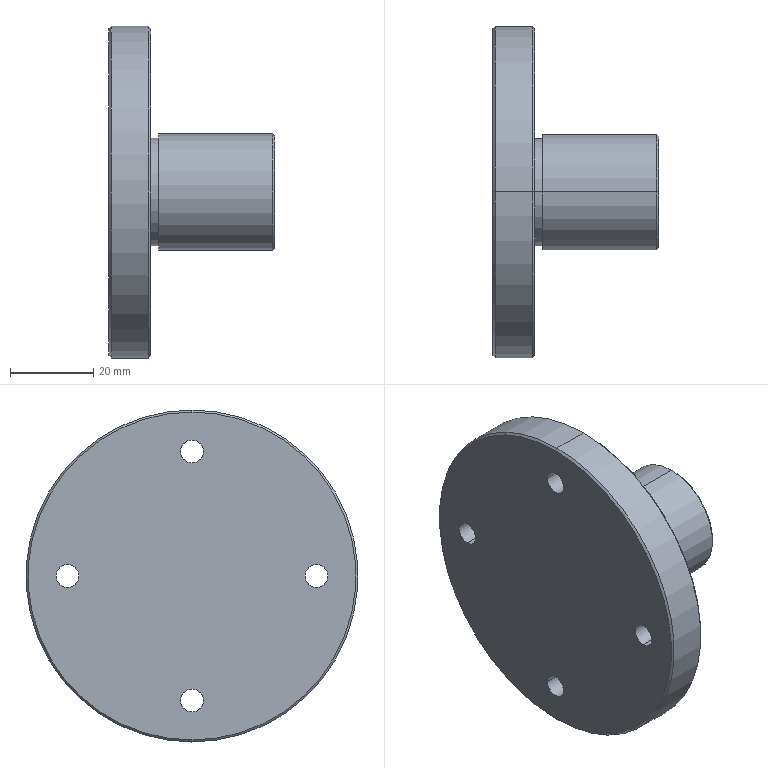Part | SolidWorks | features HoleWzd 2, Chamfer 1, CirPattern 1, ICE 1, Revolution 1 | 1 solid | 36 faces | box 40 x 80 x 80 mm | volume 66296 mm3 | cylinder 22 | plane 8 | cone 6 | commonest cylinder face diameters 5.5 x8 10 x8 26 x2 28 x2 80 x2
STEP:
#1=CARTESIAN_POINT('',(4.3,-30.,-5.));
#2=VERTEX_POINT('',#1);
#3=CARTESIAN_POINT('',(4.3,-30.,5.));
#4=VERTEX_POINT('',#3);
#5=CARTESIAN_POINT('',(4.3,-30.,0.));
#6=DIRECTION('',(1.,0.,0.));
#7=DIRECTION('',(0.,0.,1.));
#8=AXIS2_PLACEMENT_3D('',#5,#6,#7);
#9=CIRCLE('',#8,5.);
#10=EDGE_CURVE('',#2,#4,#9,.T.);
#11=ORIENTED_EDGE('',*,*,#10,.F.);
#12=CARTESIAN_POINT('',(10.,-30.,-5.));
#13=VERTEX_POINT('',#12);
#14=CARTESIAN_POINT('',(10.,-30.,-5.));
#15=DIRECTION('',(1.,0.,0.));
#16=VECTOR('',#15,1000.);
#17=LINE('',#14,#16);
#18=EDGE_CURVE('',#2,#13,#17,.T.);
#19=ORIENTED_EDGE('',*,*,#18,.T.);
#20=CARTESIAN_POINT('',(10.,-30.,5.));
#21=VERTEX_POINT('',#20);
#22=CARTESIAN_POINT('',(10.,-30.,0.));
#23=DIRECTION('',(1.,0.,0.));
#24=DIRECTION('',(0.,0.,1.));
#25=AXIS2_PLACEMENT_3D('',#22,#23,#24);
#26=CIRCLE('',#25,5.);
#27=EDGE_CURVE('',#13,#21,#26,.T.);
#28=ORIENTED_EDGE('',*,*,#27,.T.);
#29=CARTESIAN_POINT('',(10.,-30.,5.));
#30=DIRECTION('',(1.,0.,0.));
#31=VECTOR('',#30,1000.);
#32=LINE('',#29,#31);
#33=EDGE_CURVE('',#4,#21,#32,.T.);
#34=ORIENTED_EDGE('',*,*,#33,.F.);
#35=EDGE_LOOP('',(#11,#19,#28,#34));
#36=FACE_OUTER_BOUND('',#35,.T.);
#37=CARTESIAN_POINT('',(10.,-30.,0.));
#38=DIRECTION('',(1.,0.,0.));
#39=DIRECTION('',(0.,0.,1.));
#40=AXIS2_PLACEMENT_3D('',#37,#38,#39);
#41=CYLINDRICAL_SURFACE('',#40,5.);
#42=ADVANCED_FACE('',(#36),#41,.F.);
#43=CARTESIAN_POINT('',(0.,-30.,-2.75));
#44=VERTEX_POINT('',#43);
#45=CARTESIAN_POINT('',(0.,-30.,2.75));
#46=VERTEX_POINT('',#45);
#47=CARTESIAN_POINT('',(0.,-30.,0.));
#48=DIRECTION('',(1.,0.,0.));
#49=DIRECTION('',(0.,0.,1.));
#50=AXIS2_PLACEMENT_3D('',#47,#48,#49);
#51=CIRCLE('',#50,2.75);
#52=EDGE_CURVE('',#44,#46,#51,.T.);
#53=ORIENTED_EDGE('',*,*,#52,.F.);
#54=CARTESIAN_POINT('',(4.3,-30.,-2.75));
#55=VERTEX_POINT('',#54);
#56=CARTESIAN_POINT('',(10.,-30.,-2.75));
#57=DIRECTION('',(1.,0.,0.));
#58=VECTOR('',#57,1000.);
#59=LINE('',#56,#58);
#60=EDGE_CURVE('',#44,#55,#59,.T.);
#61=ORIENTED_EDGE('',*,*,#60,.T.);
#62=CARTESIAN_POINT('',(4.3,-30.,2.75));
#63=VERTEX_POINT('',#62);
#64=CARTESIAN_POINT('',(4.3,-30.,0.));
#65=DIRECTION('',(1.,0.,0.));
#66=DIRECTION('',(0.,0.,1.));
#67=AXIS2_PLACEMENT_3D('',#64,#65,#66);
#68=CIRCLE('',#67,2.75);
#69=EDGE_CURVE('',#55,#63,#68,.T.);
#70=ORIENTED_EDGE('',*,*,#69,.T.);
#71=CARTESIAN_POINT('',(10.,-30.,2.75));
#72=DIRECTION('',(1.,0.,0.));
#73=VECTOR('',#72,1000.);
#74=LINE('',#71,#73);
#75=EDGE_CURVE('',#46,#63,#74,.T.);
#76=ORIENTED_EDGE('',*,*,#75,.F.);
#77=EDGE_LOOP('',(#53,#61,#70,#76));
#78=FACE_OUTER_BOUND('',#77,.T.);
#79=CARTESIAN_POINT('',(10.,-30.,0.));
#80=DIRECTION('',(1.,0.,0.));
#81=DIRECTION('',(0.,0.,1.));
#82=AXIS2_PLACEMENT_3D('',#79,#80,#81);
#83=CYLINDRICAL_SURFACE('',#82,2.75);
#84=ADVANCED_FACE('',(#78),#83,.F.);
#85=CARTESIAN_POINT('',(4.3,5.,-30.));
#86=VERTEX_POINT('',#85);
#87=CARTESIAN_POINT('',(4.3,-5.,-30.));
#88=VERTEX_POINT('',#87);
#89=CARTESIAN_POINT('',(4.3,0.,-30.));
#90=DIRECTION('',(1.,0.,0.));
#91=DIRECTION('',(0.,-1.,0.));
#92=AXIS2_PLACEMENT_3D('',#89,#90,#91);
#93=CIRCLE('',#92,5.);
#94=EDGE_CURVE('',#86,#88,#93,.T.);
#95=ORIENTED_EDGE('',*,*,#94,.F.);
#96=CARTESIAN_POINT('',(10.,5.,-30.));
#97=VERTEX_POINT('',#96);
#98=CARTESIAN_POINT('',(10.,5.,-30.));
#99=DIRECTION('',(1.,0.,0.));
#100=VECTOR('',#99,1000.);
#101=LINE('',#98,#100);
#102=EDGE_CURVE('',#86,#97,#101,.T.);
#103=ORIENTED_EDGE('',*,*,#102,.T.);
#104=CARTESIAN_POINT('',(10.,-5.,-30.));
#105=VERTEX_POINT('',#104);
#106=CARTESIAN_POINT('',(10.,0.,-30.));
#107=DIRECTION('',(1.,0.,0.));
#108=DIRECTION('',(0.,-1.,0.));
#109=AXIS2_PLACEMENT_3D('',#106,#107,#108);
#110=CIRCLE('',#109,5.);
#111=EDGE_CURVE('',#97,#105,#110,.T.);
#112=ORIENTED_EDGE('',*,*,#111,.T.);
#113=CARTESIAN_POINT('',(10.,-5.,-30.));
#114=DIRECTION('',(1.,0.,0.));
#115=VECTOR('',#114,1000.);
#116=LINE('',#113,#115);
#117=EDGE_CURVE('',#88,#105,#116,.T.);
#118=ORIENTED_EDGE('',*,*,#117,.F.);
#119=EDGE_LOOP('',(#95,#103,#112,#118));
#120=FACE_OUTER_BOUND('',#119,.T.);
#121=CARTESIAN_POINT('',(10.,0.,-30.));
#122=DIRECTION('',(1.,0.,0.));
#123=DIRECTION('',(0.,-1.,0.));
#124=AXIS2_PLACEMENT_3D('',#121,#122,#123);
#125=CYLINDRICAL_SURFACE('',#124,5.);
#126=ADVANCED_FACE('',(#120),#125,.F.);
#127=CARTESIAN_POINT('',(0.,2.75,-30.));
#128=VERTEX_POINT('',#127);
#129=CARTESIAN_POINT('',(0.,-2.75,-30.));
#130=VERTEX_POINT('',#129);
#131=CARTESIAN_POINT('',(0.,0.,-30.));
#132=DIRECTION('',(1.,0.,0.));
#133=DIRECTION('',(0.,-1.,0.));
#134=AXIS2_PLACEMENT_3D('',#131,#132,#133);
#135=CIRCLE('',#134,2.75);
#136=EDGE_CURVE('',#128,#130,#135,.T.);
#137=ORIENTED_EDGE('',*,*,#136,.F.);
#138=CARTESIAN_POINT('',(4.3,2.75,-30.));
#139=VERTEX_POINT('',#138);
#140=CARTESIAN_POINT('',(10.,2.75,-30.));
#141=DIRECTION('',(1.,0.,0.));
#142=VECTOR('',#141,1000.);
#143=LINE('',#140,#142);
#144=EDGE_CURVE('',#128,#139,#143,.T.);
#145=ORIENTED_EDGE('',*,*,#144,.T.);
#146=CARTESIAN_POINT('',(4.3,-2.75,-30.));
#147=VERTEX_POINT('',#146);
#148=CARTESIAN_POINT('',(4.3,0.,-30.));
#149=DIRECTION('',(1.,0.,0.));
#150=DIRECTION('',(0.,-1.,0.));
#151=AXIS2_PLACEMENT_3D('',#148,#149,#150);
#152=CIRCLE('',#151,2.75);
#153=EDGE_CURVE('',#139,#147,#152,.T.);
#154=ORIENTED_EDGE('',*,*,#153,.T.);
#155=CARTESIAN_POINT('',(10.,-2.75,-30.));
#156=DIRECTION('',(1.,0.,0.));
#157=VECTOR('',#156,1000.);
#158=LINE('',#155,#157);
#159=EDGE_CURVE('',#130,#147,#158,.T.);
#160=ORIENTED_EDGE('',*,*,#159,.F.);
#161=EDGE_LOOP('',(#137,#145,#154,#160));
#162=FACE_OUTER_BOUND('',#161,.T.);
#163=CARTESIAN_POINT('',(10.,0.,-30.));
#164=DIRECTION('',(1.,0.,0.));
#165=DIRECTION('',(0.,-1.,0.));
#166=AXIS2_PLACEMENT_3D('',#163,#164,#165);
#167=CYLINDRICAL_SURFACE('',#166,2.75);
#168=ADVANCED_FACE('',(#162),#167,.F.);
#169=CARTESIAN_POINT('',(4.3,-5.,30.));
#170=VERTEX_POINT('',#169);
#171=CARTESIAN_POINT('',(4.3,5.,30.));
#172=VERTEX_POINT('',#171);
#173=CARTESIAN_POINT('',(4.3,0.,30.));
#174=DIRECTION('',(1.,0.,0.));
#175=DIRECTION('',(0.,1.,0.));
#176=AXIS2_PLACEMENT_3D('',#173,#174,#175);
#177=CIRCLE('',#176,5.);
#178=EDGE_CURVE('',#170,#172,#177,.T.);
#179=ORIENTED_EDGE('',*,*,#178,.F.);
#180=CARTESIAN_POINT('',(10.,-5.,30.));
#181=VERTEX_POINT('',#180);
#182=CARTESIAN_POINT('',(10.,-5.,30.));
#183=DIRECTION('',(1.,0.,0.));
#184=VECTOR('',#183,1000.);
#185=LINE('',#182,#184);
#186=EDGE_CURVE('',#170,#181,#185,.T.);
#187=ORIENTED_EDGE('',*,*,#186,.T.);
#188=CARTESIAN_POINT('',(10.,5.,30.));
#189=VERTEX_POINT('',#188);
#190=CARTESIAN_POINT('',(10.,0.,30.));
#191=DIRECTION('',(1.,0.,0.));
#192=DIRECTION('',(0.,1.,0.));
#193=AXIS2_PLACEMENT_3D('',#190,#191,#192);
#194=CIRCLE('',#193,5.);
#195=EDGE_CURVE('',#181,#189,#194,.T.);
#196=ORIENTED_EDGE('',*,*,#195,.T.);
#197=CARTESIAN_POINT('',(10.,5.,30.));
#198=DIRECTION('',(1.,0.,0.));
#199=VECTOR('',#198,1000.);
#200=LINE('',#197,#199);
#201=EDGE_CURVE('',#172,#189,#200,.T.);
#202=ORIENTED_EDGE('',*,*,#201,.F.);
#203=EDGE_LOOP('',(#179,#187,#196,#202));
#204=FACE_OUTER_BOUND('',#203,.T.);
#205=CARTESIAN_POINT('',(10.,0.,30.));
#206=DIRECTION('',(1.,0.,0.));
#207=DIRECTION('',(0.,1.,0.));
#208=AXIS2_PLACEMENT_3D('',#205,#206,#207);
#209=CYLINDRICAL_SURFACE('',#208,5.);
#210=ADVANCED_FACE('',(#204),#209,.F.);
#211=CARTESIAN_POINT('',(0.,-2.75,30.));
#212=VERTEX_POINT('',#211);
#213=CARTESIAN_POINT('',(0.,2.75,30.));
#214=VERTEX_POINT('',#213);
#215=CARTESIAN_POINT('',(0.,0.,30.));
#216=DIRECTION('',(1.,0.,0.));
#217=DIRECTION('',(0.,1.,0.));
#218=AXIS2_PLACEMENT_3D('',#215,#216,#217);
#219=CIRCLE('',#218,2.75);
#220=EDGE_CURVE('',#212,#214,#219,.T.);
#221=ORIENTED_EDGE('',*,*,#220,.F.);
#222=CARTESIAN_POINT('',(4.3,-2.75,30.));
#223=VERTEX_POINT('',#222);
#224=CARTESIAN_POINT('',(10.,-2.75,30.));
#225=DIRECTION('',(1.,0.,0.));
#226=VECTOR('',#225,1000.);
#227=LINE('',#224,#226);
#228=EDGE_CURVE('',#212,#223,#227,.T.);
#229=ORIENTED_EDGE('',*,*,#228,.T.);
#230=CARTESIAN_POINT('',(4.3,2.75,30.));
#231=VERTEX_POINT('',#230);
#232=CARTESIAN_POINT('',(4.3,0.,30.));
#233=DIRECTION('',(1.,0.,0.));
#234=DIRECTION('',(0.,1.,0.));
#235=AXIS2_PLACEMENT_3D('',#232,#233,#234);
#236=CIRCLE('',#235,2.75);
#237=EDGE_CURVE('',#223,#231,#236,.T.);
#238=ORIENTED_EDGE('',*,*,#237,.T.);
#239=CARTESIAN_POINT('',(10.,2.75,30.));
#240=DIRECTION('',(1.,0.,0.));
#241=VECTOR('',#240,1000.);
#242=LINE('',#239,#241);
#243=EDGE_CURVE('',#214,#231,#242,.T.);
#244=ORIENTED_EDGE('',*,*,#243,.F.);
#245=EDGE_LOOP('',(#221,#229,#238,#244));
#246=FACE_OUTER_BOUND('',#245,.T.);
#247=CARTESIAN_POINT('',(10.,0.,30.));
#248=DIRECTION('',(1.,0.,0.));
#249=DIRECTION('',(0.,1.,0.));
#250=AXIS2_PLACEMENT_3D('',#247,#248,#249);
#251=CYLINDRICAL_SURFACE('',#250,2.75);
#252=ADVANCED_FACE('',(#246),#251,.F.);
#253=CARTESIAN_POINT('',(4.3,30.,5.));
#254=VERTEX_POINT('',#253);
#255=CARTESIAN_POINT('',(4.3,30.,-5.));
#256=VERTEX_POINT('',#255);
#257=CARTESIAN_POINT('',(4.3,30.,0.));
#258=DIRECTION('',(1.,0.,0.));
#259=DIRECTION('',(0.,0.,-1.));
#260=AXIS2_PLACEMENT_3D('',#257,#258,#259);
#261=CIRCLE('',#260,5.);
#262=EDGE_CURVE('',#254,#256,#261,.T.);
#263=ORIENTED_EDGE('',*,*,#262,.F.);
#264=CARTESIAN_POINT('',(10.,30.,5.));
#265=VERTEX_POINT('',#264);
#266=CARTESIAN_POINT('',(10.,30.,5.));
#267=DIRECTION('',(1.,0.,0.));
#268=VECTOR('',#267,1000.);
#269=LINE('',#266,#268);
#270=EDGE_CURVE('',#254,#265,#269,.T.);
#271=ORIENTED_EDGE('',*,*,#270,.T.);
#272=CARTESIAN_POINT('',(10.,30.,-5.));
#273=VERTEX_POINT('',#272);
#274=CARTESIAN_POINT('',(10.,30.,0.));
#275=DIRECTION('',(1.,0.,0.));
#276=DIRECTION('',(0.,0.,-1.));
#277=AXIS2_PLACEMENT_3D('',#274,#275,#276);
#278=CIRCLE('',#277,5.);
#279=EDGE_CURVE('',#265,#273,#278,.T.);
#280=ORIENTED_EDGE('',*,*,#279,.T.);
#281=CARTESIAN_POINT('',(10.,30.,-5.));
#282=DIRECTION('',(1.,0.,0.));
#283=VECTOR('',#282,1000.);
#284=LINE('',#281,#283);
#285=EDGE_CURVE('',#256,#273,#284,.T.);
#286=ORIENTED_EDGE('',*,*,#285,.F.);
#287=EDGE_LOOP('',(#263,#271,#280,#286));
#288=FACE_OUTER_BOUND('',#287,.T.);
#289=CARTESIAN_POINT('',(10.,30.,0.));
#290=DIRECTION('',(1.,0.,0.));
#291=DIRECTION('',(0.,0.,-1.));
#292=AXIS2_PLACEMENT_3D('',#289,#290,#291);
#293=CYLINDRICAL_SURFACE('',#292,5.);
#294=ADVANCED_FACE('',(#288),#293,.F.);
#295=CARTESIAN_POINT('',(0.,30.,2.75));
#296=VERTEX_POINT('',#295);
#297=CARTESIAN_POINT('',(0.,30.,-2.75));
#298=VERTEX_POINT('',#297);
#299=CARTESIAN_POINT('',(0.,30.,0.));
#300=DIRECTION('',(1.,0.,0.));
#301=DIRECTION('',(0.,0.,-1.));
#302=AXIS2_PLACEMENT_3D('',#299,#300,#301);
#303=CIRCLE('',#302,2.75);
#304=EDGE_CURVE('',#296,#298,#303,.T.);
#305=ORIENTED_EDGE('',*,*,#304,.F.);
#306=CARTESIAN_POINT('',(4.3,30.,2.75));
#307=VERTEX_POINT('',#306);
#308=CARTESIAN_POINT('',(10.,30.,2.75));
#309=DIRECTION('',(1.,0.,0.));
#310=VECTOR('',#309,1000.);
#311=LINE('',#308,#310);
#312=EDGE_CURVE('',#296,#307,#311,.T.);
#313=ORIENTED_EDGE('',*,*,#312,.T.);
#314=CARTESIAN_POINT('',(4.3,30.,-2.75));
#315=VERTEX_POINT('',#314);
#316=CARTESIAN_POINT('',(4.3,30.,0.));
#317=DIRECTION('',(1.,0.,0.));
#318=DIRECTION('',(0.,0.,-1.));
#319=AXIS2_PLACEMENT_3D('',#316,#317,#318);
#320=CIRCLE('',#319,2.75);
#321=EDGE_CURVE('',#307,#315,#320,.T.);
#322=ORIENTED_EDGE('',*,*,#321,.T.);
#323=CARTESIAN_POINT('',(10.,30.,-2.75));
#324=DIRECTION('',(1.,0.,0.));
#325=VECTOR('',#324,1000.);
#326=LINE('',#323,#325);
#327=EDGE_CURVE('',#298,#315,#326,.T.);
#328=ORIENTED_EDGE('',*,*,#327,.F.);
#329=EDGE_LOOP('',(#305,#313,#322,#328));
#330=FACE_OUTER_BOUND('',#329,.T.);
#331=CARTESIAN_POINT('',(10.,30.,0.));
#332=DIRECTION('',(1.,0.,0.));
#333=DIRECTION('',(0.,0.,-1.));
#334=AXIS2_PLACEMENT_3D('',#331,#332,#333);
#335=CYLINDRICAL_SURFACE('',#334,2.75);
#336=ADVANCED_FACE('',(#330),#335,.F.);
#337=CARTESIAN_POINT('',(40.,0.,-13.5));
#338=VERTEX_POINT('',#337);
#339=CARTESIAN_POINT('',(40.,0.,13.5));
#340=VERTEX_POINT('',#339);
#341=CARTESIAN_POINT('',(40.,0.,0.));
#342=DIRECTION('',(1.,0.,0.));
#343=DIRECTION('',(0.,0.,1.));
#344=AXIS2_PLACEMENT_3D('',#341,#342,#343);
#345=CIRCLE('',#344,13.5);
#346=EDGE_CURVE('',#338,#340,#345,.T.);
#347=ORIENTED_EDGE('',*,*,#346,.F.);
#348=CARTESIAN_POINT('',(39.5,0.,-14.));
#349=VERTEX_POINT('',#348);
#350=CARTESIAN_POINT('',(39.5,0.,-14.));
#351=DIRECTION('',(-0.7071,0.,-0.7071));
#352=VECTOR('',#351,1000.);
#353=LINE('',#350,#352);
#354=EDGE_CURVE('',#338,#349,#353,.T.);
#355=ORIENTED_EDGE('',*,*,#354,.T.);
#356=CARTESIAN_POINT('',(39.5,0.,14.));
#357=VERTEX_POINT('',#356);
#358=CARTESIAN_POINT('',(39.5,0.,0.));
#359=DIRECTION('',(-1.,0.,0.));
#360=DIRECTION('',(0.,0.,1.));
#361=AXIS2_PLACEMENT_3D('',#358,#359,#360);
#362=CIRCLE('',#361,14.);
#363=EDGE_CURVE('',#357,#349,#362,.T.);
#364=ORIENTED_EDGE('',*,*,#363,.F.);
#365=CARTESIAN_POINT('',(39.5,0.,14.));
#366=DIRECTION('',(-0.7071,0.,0.7071));
#367=VECTOR('',#366,1000.);
#368=LINE('',#365,#367);
#369=EDGE_CURVE('',#340,#357,#368,.T.);
#370=ORIENTED_EDGE('',*,*,#369,.F.);
#371=EDGE_LOOP('',(#347,#355,#364,#370));
#372=FACE_OUTER_BOUND('',#371,.T.);
#373=CARTESIAN_POINT('',(39.5,0.,0.));
#374=DIRECTION('',(-1.,0.,0.));
#375=DIRECTION('',(0.,0.,1.));
#376=AXIS2_PLACEMENT_3D('',#373,#374,#375);
#377=CONICAL_SURFACE('',#376,14.,0.7854);
#378=ADVANCED_FACE('',(#372),#377,.T.);
#379=CARTESIAN_POINT('',(0.,0.,39.5));
#380=VERTEX_POINT('',#379);
#381=CARTESIAN_POINT('',(0.,0.,-39.5));
#382=VERTEX_POINT('',#381);
#383=CARTESIAN_POINT('',(0.,0.,0.));
#384=DIRECTION('',(-1.,0.,0.));
#385=DIRECTION('',(0.,0.,-1.));
#386=AXIS2_PLACEMENT_3D('',#383,#384,#385);
#387=CIRCLE('',#386,39.5);
#388=EDGE_CURVE('',#380,#382,#387,.T.);
#389=ORIENTED_EDGE('',*,*,#388,.F.);
#390=CARTESIAN_POINT('',(0.5,0.,40.));
#391=VERTEX_POINT('',#390);
#392=CARTESIAN_POINT('',(0.,0.,39.5));
#393=DIRECTION('',(0.7071,0.,0.7071));
#394=VECTOR('',#393,1000.);
#395=LINE('',#392,#394);
#396=EDGE_CURVE('',#380,#391,#395,.T.);
#397=ORIENTED_EDGE('',*,*,#396,.T.);
#398=CARTESIAN_POINT('',(0.5,0.,-40.));
#399=VERTEX_POINT('',#398);
#400=CARTESIAN_POINT('',(0.5,0.,0.));
#401=DIRECTION('',(1.,0.,0.));
#402=DIRECTION('',(0.,0.,-1.));
#403=AXIS2_PLACEMENT_3D('',#400,#401,#402);
#404=CIRCLE('',#403,40.);
#405=EDGE_CURVE('',#399,#391,#404,.T.);
#406=ORIENTED_EDGE('',*,*,#405,.F.);
#407=CARTESIAN_POINT('',(0.,0.,-39.5));
#408=DIRECTION('',(0.7071,0.,-0.7071));
#409=VECTOR('',#408,1000.);
#410=LINE('',#407,#409);
#411=EDGE_CURVE('',#382,#399,#410,.T.);
#412=ORIENTED_EDGE('',*,*,#411,.F.);
#413=EDGE_LOOP('',(#389,#397,#406,#412));
#414=FACE_OUTER_BOUND('',#413,.T.);
#415=CARTESIAN_POINT('',(0.,0.,0.));
#416=DIRECTION('',(1.,0.,0.));
#417=DIRECTION('',(0.,0.,-1.));
#418=AXIS2_PLACEMENT_3D('',#415,#416,#417);
#419=CONICAL_SURFACE('',#418,39.5,0.7854);
#420=ADVANCED_FACE('',(#414),#419,.T.);
#421=CARTESIAN_POINT('',(10.,0.,-39.5));
#422=VERTEX_POINT('',#421);
#423=CARTESIAN_POINT('',(10.,0.,39.5));
#424=VERTEX_POINT('',#423);
#425=CARTESIAN_POINT('',(10.,0.,0.));
#426=DIRECTION('',(1.,0.,0.));
#427=DIRECTION('',(0.,0.,1.));
#428=AXIS2_PLACEMENT_3D('',#425,#426,#427);
#429=CIRCLE('',#428,39.5);
#430=EDGE_CURVE('',#422,#424,#429,.T.);
#431=ORIENTED_EDGE('',*,*,#430,.F.);
#432=CARTESIAN_POINT('',(9.5,0.,-40.));
#433=VERTEX_POINT('',#432);
#434=CARTESIAN_POINT('',(9.5,0.,-40.));
#435=DIRECTION('',(-0.7071,0.,-0.7071));
#436=VECTOR('',#435,1000.);
#437=LINE('',#434,#436);
#438=EDGE_CURVE('',#422,#433,#437,.T.);
#439=ORIENTED_EDGE('',*,*,#438,.T.);
#440=CARTESIAN_POINT('',(9.5,0.,40.));
#441=VERTEX_POINT('',#440);
#442=CARTESIAN_POINT('',(9.5,0.,0.));
#443=DIRECTION('',(-1.,0.,0.));
#444=DIRECTION('',(0.,0.,1.));
#445=AXIS2_PLACEMENT_3D('',#442,#443,#444);
#446=CIRCLE('',#445,40.);
#447=EDGE_CURVE('',#441,#433,#446,.T.);
#448=ORIENTED_EDGE('',*,*,#447,.F.);
#449=CARTESIAN_POINT('',(9.5,0.,40.));
#450=DIRECTION('',(-0.7071,0.,0.7071));
#451=VECTOR('',#450,1000.);
#452=LINE('',#449,#451);
#453=EDGE_CURVE('',#424,#441,#452,.T.);
#454=ORIENTED_EDGE('',*,*,#453,.F.);
#455=EDGE_LOOP('',(#431,#439,#448,#454));
#456=FACE_OUTER_BOUND('',#455,.T.);
#457=CARTESIAN_POINT('',(9.5,0.,0.));
#458=DIRECTION('',(-1.,0.,0.));
#459=DIRECTION('',(0.,0.,1.));
#460=AXIS2_PLACEMENT_3D('',#457,#458,#459);
#461=CONICAL_SURFACE('',#460,40.,0.7854);
#462=ADVANCED_FACE('',(#456),#461,.T.);
#463=ORIENTED_EDGE('',*,*,#363,.T.);
#464=CARTESIAN_POINT('',(12.,0.,-14.));
#465=VERTEX_POINT('',#464);
#466=CARTESIAN_POINT('',(0.,0.,-14.));
#467=DIRECTION('',(-1.,0.,0.));
#468=VECTOR('',#467,1000.);
#469=LINE('',#466,#468);
#470=EDGE_CURVE('',#349,#465,#469,.T.);
#471=ORIENTED_EDGE('',*,*,#470,.T.);
#472=CARTESIAN_POINT('',(12.,0.,14.));
#473=VERTEX_POINT('',#472);
#474=CARTESIAN_POINT('',(12.,0.,0.));
#475=DIRECTION('',(-1.,0.,0.));
#476=DIRECTION('',(0.,0.,1.));
#477=AXIS2_PLACEMENT_3D('',#474,#475,#476);
#478=CIRCLE('',#477,14.);
#479=EDGE_CURVE('',#473,#465,#478,.T.);
#480=ORIENTED_EDGE('',*,*,#479,.F.);
#481=CARTESIAN_POINT('',(0.,0.,14.));
#482=DIRECTION('',(-1.,0.,0.));
#483=VECTOR('',#482,1000.);
#484=LINE('',#481,#483);
#485=EDGE_CURVE('',#357,#473,#484,.T.);
#486=ORIENTED_EDGE('',*,*,#485,.F.);
#487=EDGE_LOOP('',(#463,#471,#480,#486));
#488=FACE_OUTER_BOUND('',#487,.T.);
#489=CARTESIAN_POINT('',(0.,0.,0.));
#490=DIRECTION('',(-1.,0.,0.));
#491=DIRECTION('',(0.,0.,1.));
#492=AXIS2_PLACEMENT_3D('',#489,#490,#491);
#493=CYLINDRICAL_SURFACE('',#492,14.);
#494=ADVANCED_FACE('',(#488),#493,.T.);
#495=CARTESIAN_POINT('',(12.,0.,13.));
#496=VERTEX_POINT('',#495);
#497=CARTESIAN_POINT('',(12.,0.,-13.));
#498=VERTEX_POINT('',#497);
#499=CARTESIAN_POINT('',(12.,0.,0.));
#500=DIRECTION('',(-1.,0.,0.));
#501=DIRECTION('',(0.,0.,1.));
#502=AXIS2_PLACEMENT_3D('',#499,#500,#501);
#503=CIRCLE('',#502,13.);
#504=EDGE_CURVE('',#496,#498,#503,.T.);
#505=ORIENTED_EDGE('',*,*,#504,.T.);
#506=CARTESIAN_POINT('',(10.,0.,-13.));
#507=VERTEX_POINT('',#506);
#508=CARTESIAN_POINT('',(0.,0.,-13.));
#509=DIRECTION('',(-1.,0.,0.));
#510=VECTOR('',#509,1000.);
#511=LINE('',#508,#510);
#512=EDGE_CURVE('',#498,#507,#511,.T.);
#513=ORIENTED_EDGE('',*,*,#512,.T.);
#514=CARTESIAN_POINT('',(10.,0.,13.));
#515=VERTEX_POINT('',#514);
#516=CARTESIAN_POINT('',(10.,0.,0.));
#517=DIRECTION('',(-1.,0.,0.));
#518=DIRECTION('',(0.,0.,1.));
#519=AXIS2_PLACEMENT_3D('',#516,#517,#518);
#520=CIRCLE('',#519,13.);
#521=EDGE_CURVE('',#515,#507,#520,.T.);
#522=ORIENTED_EDGE('',*,*,#521,.F.);
#523=CARTESIAN_POINT('',(0.,0.,13.));
#524=DIRECTION('',(-1.,0.,0.));
#525=VECTOR('',#524,1000.);
#526=LINE('',#523,#525);
#527=EDGE_CURVE('',#496,#515,#526,.T.);
#528=ORIENTED_EDGE('',*,*,#527,.F.);
#529=EDGE_LOOP('',(#505,#513,#522,#528));
#530=FACE_OUTER_BOUND('',#529,.T.);
#531=CARTESIAN_POINT('',(0.,0.,0.));
#532=DIRECTION('',(-1.,0.,0.));
#533=DIRECTION('',(0.,0.,1.));
#534=AXIS2_PLACEMENT_3D('',#531,#532,#533);
#535=CYLINDRICAL_SURFACE('',#534,13.);
#536=ADVANCED_FACE('',(#530),#535,.T.);
#537=ORIENTED_EDGE('',*,*,#447,.T.);
#538=CARTESIAN_POINT('',(0.,0.,-40.));
#539=DIRECTION('',(-1.,0.,0.));
#540=VECTOR('',#539,1000.);
#541=LINE('',#538,#540);
#542=EDGE_CURVE('',#433,#399,#541,.T.);
#543=ORIENTED_EDGE('',*,*,#542,.T.);
#544=ORIENTED_EDGE('',*,*,#405,.T.);
#545=CARTESIAN_POINT('',(0.,0.,40.));
#546=DIRECTION('',(-1.,0.,0.));
#547=VECTOR('',#546,1000.);
#548=LINE('',#545,#547);
#549=EDGE_CURVE('',#441,#391,#548,.T.);
#550=ORIENTED_EDGE('',*,*,#549,.F.);
#551=EDGE_LOOP('',(#537,#543,#544,#550));
#552=FACE_OUTER_BOUND('',#551,.T.);
#553=CARTESIAN_POINT('',(0.,0.,0.));
#554=DIRECTION('',(-1.,0.,0.));
#555=DIRECTION('',(0.,0.,1.));
#556=AXIS2_PLACEMENT_3D('',#553,#554,#555);
#557=CYLINDRICAL_SURFACE('',#556,40.);
#558=ADVANCED_FACE('',(#552),#557,.T.);
#559=CARTESIAN_POINT('',(0.,-30.,0.));
#560=DIRECTION('',(1.,0.,0.));
#561=DIRECTION('',(0.,0.,1.));
#562=AXIS2_PLACEMENT_3D('',#559,#560,#561);
#563=CIRCLE('',#562,2.75);
#564=EDGE_CURVE('',#46,#44,#563,.T.);
#565=ORIENTED_EDGE('',*,*,#564,.T.);
#566=ORIENTED_EDGE('',*,*,#52,.T.);
#567=EDGE_LOOP('',(#565,#566));
#568=FACE_BOUND('',#567,.T.);
#569=CARTESIAN_POINT('',(0.,0.,-30.));
#570=DIRECTION('',(1.,0.,0.));
#571=DIRECTION('',(0.,-1.,0.));
#572=AXIS2_PLACEMENT_3D('',#569,#570,#571);
#573=CIRCLE('',#572,2.75);
#574=EDGE_CURVE('',#130,#128,#573,.T.);
#575=ORIENTED_EDGE('',*,*,#574,.T.);
#576=ORIENTED_EDGE('',*,*,#136,.T.);
#577=EDGE_LOOP('',(#575,#576));
#578=FACE_BOUND('',#577,.T.);
#579=CARTESIAN_POINT('',(0.,0.,30.));
#580=DIRECTION('',(1.,0.,0.));
#581=DIRECTION('',(0.,1.,0.));
#582=AXIS2_PLACEMENT_3D('',#579,#580,#581);
#583=CIRCLE('',#582,2.75);
#584=EDGE_CURVE('',#214,#212,#583,.T.);
#585=ORIENTED_EDGE('',*,*,#584,.T.);
#586=ORIENTED_EDGE('',*,*,#220,.T.);
#587=EDGE_LOOP('',(#585,#586));
#588=FACE_BOUND('',#587,.T.);
#589=CARTESIAN_POINT('',(0.,30.,0.));
#590=DIRECTION('',(1.,0.,0.));
#591=DIRECTION('',(0.,0.,-1.));
#592=AXIS2_PLACEMENT_3D('',#589,#590,#591);
#593=CIRCLE('',#592,2.75);
#594=EDGE_CURVE('',#298,#296,#593,.T.);
#595=ORIENTED_EDGE('',*,*,#594,.T.);
#596=ORIENTED_EDGE('',*,*,#304,.T.);
#597=EDGE_LOOP('',(#595,#596));
#598=FACE_BOUND('',#597,.T.);
#599=CARTESIAN_POINT('',(0.,0.,0.));
#600=DIRECTION('',(-1.,0.,0.));
#601=DIRECTION('',(0.,0.,-1.));
#602=AXIS2_PLACEMENT_3D('',#599,#600,#601);
#603=CIRCLE('',#602,39.5);
#604=EDGE_CURVE('',#382,#380,#603,.T.);
#605=ORIENTED_EDGE('',*,*,#604,.T.);
#606=ORIENTED_EDGE('',*,*,#388,.T.);
#607=EDGE_LOOP('',(#605,#606));
#608=FACE_OUTER_BOUND('',#607,.T.);
#609=CARTESIAN_POINT('',(0.,0.,0.));
#610=DIRECTION('',(1.,0.,0.));
#611=DIRECTION('',(0.,0.,-1.));
#612=AXIS2_PLACEMENT_3D('',#609,#610,#611);
#613=PLANE('',#612);
#614=ADVANCED_FACE('',(#568,#578,#588,#598,#608),#613,.F.);
#615=ORIENTED_EDGE('',*,*,#542,.F.);
#616=CARTESIAN_POINT('',(9.5,0.,0.));
#617=DIRECTION('',(-1.,0.,0.));
#618=DIRECTION('',(0.,0.,1.));
#619=AXIS2_PLACEMENT_3D('',#616,#617,#618);
#620=CIRCLE('',#619,40.);
#621=EDGE_CURVE('',#433,#441,#620,.T.);
#622=ORIENTED_EDGE('',*,*,#621,.T.);
#623=ORIENTED_EDGE('',*,*,#549,.T.);
#624=CARTESIAN_POINT('',(0.5,0.,0.));
#625=DIRECTION('',(1.,0.,0.));
#626=DIRECTION('',(0.,0.,-1.));
#627=AXIS2_PLACEMENT_3D('',#624,#625,#626);
#628=CIRCLE('',#627,40.);
#629=EDGE_CURVE('',#391,#399,#628,.T.);
#630=ORIENTED_EDGE('',*,*,#629,.T.);
#631=EDGE_LOOP('',(#615,#622,#623,#630));
#632=FACE_OUTER_BOUND('',#631,.T.);
#633=CARTESIAN_POINT('',(0.,0.,0.));
#634=DIRECTION('',(-1.,0.,0.));
#635=DIRECTION('',(0.,0.,1.));
#636=AXIS2_PLACEMENT_3D('',#633,#634,#635);
#637=CYLINDRICAL_SURFACE('',#636,40.);
#638=ADVANCED_FACE('',(#632),#637,.T.);
#639=CARTESIAN_POINT('',(10.,-30.,0.));
#640=DIRECTION('',(1.,0.,0.));
#641=DIRECTION('',(0.,0.,1.));
#642=AXIS2_PLACEMENT_3D('',#639,#640,#641);
#643=CIRCLE('',#642,5.);
#644=EDGE_CURVE('',#21,#13,#643,.T.);
#645=ORIENTED_EDGE('',*,*,#644,.F.);
#646=ORIENTED_EDGE('',*,*,#27,.F.);
#647=EDGE_LOOP('',(#645,#646));
#648=FACE_BOUND('',#647,.T.);
#649=CARTESIAN_POINT('',(10.,0.,-30.));
#650=DIRECTION('',(1.,0.,0.));
#651=DIRECTION('',(0.,-1.,0.));
#652=AXIS2_PLACEMENT_3D('',#649,#650,#651);
#653=CIRCLE('',#652,5.);
#654=EDGE_CURVE('',#105,#97,#653,.T.);
#655=ORIENTED_EDGE('',*,*,#654,.F.);
#656=ORIENTED_EDGE('',*,*,#111,.F.);
#657=EDGE_LOOP('',(#655,#656));
#658=FACE_BOUND('',#657,.T.);
#659=CARTESIAN_POINT('',(10.,0.,30.));
#660=DIRECTION('',(1.,0.,0.));
#661=DIRECTION('',(0.,1.,0.));
#662=AXIS2_PLACEMENT_3D('',#659,#660,#661);
#663=CIRCLE('',#662,5.);
#664=EDGE_CURVE('',#189,#181,#663,.T.);
#665=ORIENTED_EDGE('',*,*,#664,.F.);
#666=ORIENTED_EDGE('',*,*,#195,.F.);
#667=EDGE_LOOP('',(#665,#666));
#668=FACE_BOUND('',#667,.T.);
#669=CARTESIAN_POINT('',(10.,30.,0.));
#670=DIRECTION('',(1.,0.,0.));
#671=DIRECTION('',(0.,0.,-1.));
#672=AXIS2_PLACEMENT_3D('',#669,#670,#671);
#673=CIRCLE('',#672,5.);
#674=EDGE_CURVE('',#273,#265,#673,.T.);
#675=ORIENTED_EDGE('',*,*,#674,.F.);
#676=ORIENTED_EDGE('',*,*,#279,.F.);
#677=EDGE_LOOP('',(#675,#676));
#678=FACE_BOUND('',#677,.T.);
#679=CARTESIAN_POINT('',(10.,0.,0.));
#680=DIRECTION('',(1.,0.,0.));
#681=DIRECTION('',(0.,0.,1.));
#682=AXIS2_PLACEMENT_3D('',#679,#680,#681);
#683=CIRCLE('',#682,39.5);
#684=EDGE_CURVE('',#424,#422,#683,.T.);
#685=ORIENTED_EDGE('',*,*,#684,.T.);
#686=ORIENTED_EDGE('',*,*,#430,.T.);
#687=EDGE_LOOP('',(#685,#686));
#688=FACE_OUTER_BOUND('',#687,.T.);
#689=ORIENTED_EDGE('',*,*,#521,.T.);
#690=CARTESIAN_POINT('',(10.,0.,0.));
#691=DIRECTION('',(-1.,0.,0.));
#692=DIRECTION('',(0.,0.,1.));
#693=AXIS2_PLACEMENT_3D('',#690,#691,#692);
#694=CIRCLE('',#693,13.);
#695=EDGE_CURVE('',#507,#515,#694,.T.);
#696=ORIENTED_EDGE('',*,*,#695,.T.);
#697=EDGE_LOOP('',(#689,#696));
#698=FACE_BOUND('',#697,.T.);
#699=CARTESIAN_POINT('',(10.,40.,0.));
#700=DIRECTION('',(-1.,0.,0.));
#701=DIRECTION('',(0.,0.,1.));
#702=AXIS2_PLACEMENT_3D('',#699,#700,#701);
#703=PLANE('',#702);
#704=ADVANCED_FACE('',(#648,#658,#668,#678,#688,#698),#703,.F.);
#705=ORIENTED_EDGE('',*,*,#512,.F.);
#706=CARTESIAN_POINT('',(12.,0.,0.));
#707=DIRECTION('',(-1.,0.,0.));
#708=DIRECTION('',(0.,0.,1.));
#709=AXIS2_PLACEMENT_3D('',#706,#707,#708);
#710=CIRCLE('',#709,13.);
#711=EDGE_CURVE('',#498,#496,#710,.T.);
#712=ORIENTED_EDGE('',*,*,#711,.T.);
#713=ORIENTED_EDGE('',*,*,#527,.T.);
#714=ORIENTED_EDGE('',*,*,#695,.F.);
#715=EDGE_LOOP('',(#705,#712,#713,#714));
#716=FACE_OUTER_BOUND('',#715,.T.);
#717=CARTESIAN_POINT('',(0.,0.,0.));
#718=DIRECTION('',(-1.,0.,0.));
#719=DIRECTION('',(0.,0.,1.));
#720=AXIS2_PLACEMENT_3D('',#717,#718,#719);
#721=CYLINDRICAL_SURFACE('',#720,13.);
#722=ADVANCED_FACE('',(#716),#721,.T.);
#723=ORIENTED_EDGE('',*,*,#504,.F.);
#724=ORIENTED_EDGE('',*,*,#711,.F.);
#725=EDGE_LOOP('',(#723,#724));
#726=FACE_BOUND('',#725,.T.);
#727=ORIENTED_EDGE('',*,*,#479,.T.);
#728=CARTESIAN_POINT('',(12.,0.,0.));
#729=DIRECTION('',(-1.,0.,0.));
#730=DIRECTION('',(0.,0.,1.));
#731=AXIS2_PLACEMENT_3D('',#728,#729,#730);
#732=CIRCLE('',#731,14.);
#733=EDGE_CURVE('',#465,#473,#732,.T.);
#734=ORIENTED_EDGE('',*,*,#733,.T.);
#735=EDGE_LOOP('',(#727,#734));
#736=FACE_OUTER_BOUND('',#735,.T.);
#737=CARTESIAN_POINT('',(12.,13.,0.));
#738=DIRECTION('',(1.,0.,0.));
#739=DIRECTION('',(0.,0.,-1.));
#740=AXIS2_PLACEMENT_3D('',#737,#738,#739);
#741=PLANE('',#740);
#742=ADVANCED_FACE('',(#726,#736),#741,.F.);
#743=ORIENTED_EDGE('',*,*,#470,.F.);
#744=CARTESIAN_POINT('',(39.5,0.,0.));
#745=DIRECTION('',(-1.,0.,0.));
#746=DIRECTION('',(0.,0.,1.));
#747=AXIS2_PLACEMENT_3D('',#744,#745,#746);
#748=CIRCLE('',#747,14.);
#749=EDGE_CURVE('',#349,#357,#748,.T.);
#750=ORIENTED_EDGE('',*,*,#749,.T.);
#751=ORIENTED_EDGE('',*,*,#485,.T.);
#752=ORIENTED_EDGE('',*,*,#733,.F.);
#753=EDGE_LOOP('',(#743,#750,#751,#752));
#754=FACE_OUTER_BOUND('',#753,.T.);
#755=CARTESIAN_POINT('',(0.,0.,0.));
#756=DIRECTION('',(-1.,0.,0.));
#757=DIRECTION('',(0.,0.,1.));
#758=AXIS2_PLACEMENT_3D('',#755,#756,#757);
#759=CYLINDRICAL_SURFACE('',#758,14.);
#760=ADVANCED_FACE('',(#754),#759,.T.);
#761=CARTESIAN_POINT('',(40.,0.,0.));
#762=DIRECTION('',(1.,0.,0.));
#763=DIRECTION('',(0.,0.,1.));
#764=AXIS2_PLACEMENT_3D('',#761,#762,#763);
#765=CIRCLE('',#764,13.5);
#766=EDGE_CURVE('',#340,#338,#765,.T.);
#767=ORIENTED_EDGE('',*,*,#766,.T.);
#768=ORIENTED_EDGE('',*,*,#346,.T.);
#769=EDGE_LOOP('',(#767,#768));
#770=FACE_OUTER_BOUND('',#769,.T.);
#771=CARTESIAN_POINT('',(40.,14.,0.));
#772=DIRECTION('',(-1.,0.,0.));
#773=DIRECTION('',(0.,0.,1.));
#774=AXIS2_PLACEMENT_3D('',#771,#772,#773);
#775=PLANE('',#774);
#776=ADVANCED_FACE('',(#770),#775,.F.);
#777=ORIENTED_EDGE('',*,*,#438,.F.);
#778=ORIENTED_EDGE('',*,*,#684,.F.);
#779=ORIENTED_EDGE('',*,*,#453,.T.);
#780=ORIENTED_EDGE('',*,*,#621,.F.);
#781=EDGE_LOOP('',(#777,#778,#779,#780));
#782=FACE_OUTER_BOUND('',#781,.T.);
#783=CARTESIAN_POINT('',(9.5,0.,0.));
#784=DIRECTION('',(-1.,0.,0.));
#785=DIRECTION('',(0.,0.,1.));
#786=AXIS2_PLACEMENT_3D('',#783,#784,#785);
#787=CONICAL_SURFACE('',#786,40.,0.7854);
#788=ADVANCED_FACE('',(#782),#787,.T.);
#789=ORIENTED_EDGE('',*,*,#396,.F.);
#790=ORIENTED_EDGE('',*,*,#604,.F.);
#791=ORIENTED_EDGE('',*,*,#411,.T.);
#792=ORIENTED_EDGE('',*,*,#629,.F.);
#793=EDGE_LOOP('',(#789,#790,#791,#792));
#794=FACE_OUTER_BOUND('',#793,.T.);
#795=CARTESIAN_POINT('',(0.,0.,0.));
#796=DIRECTION('',(1.,0.,0.));
#797=DIRECTION('',(0.,0.,-1.));
#798=AXIS2_PLACEMENT_3D('',#795,#796,#797);
#799=CONICAL_SURFACE('',#798,39.5,0.7854);
#800=ADVANCED_FACE('',(#794),#799,.T.);
#801=ORIENTED_EDGE('',*,*,#354,.F.);
#802=ORIENTED_EDGE('',*,*,#766,.F.);
#803=ORIENTED_EDGE('',*,*,#369,.T.);
#804=ORIENTED_EDGE('',*,*,#749,.F.);
#805=EDGE_LOOP('',(#801,#802,#803,#804));
#806=FACE_OUTER_BOUND('',#805,.T.);
#807=CARTESIAN_POINT('',(39.5,0.,0.));
#808=DIRECTION('',(-1.,0.,0.));
#809=DIRECTION('',(0.,0.,1.));
#810=AXIS2_PLACEMENT_3D('',#807,#808,#809);
#811=CONICAL_SURFACE('',#810,14.,0.7854);
#812=ADVANCED_FACE('',(#806),#811,.T.);
#813=ORIENTED_EDGE('',*,*,#312,.F.);
#814=ORIENTED_EDGE('',*,*,#594,.F.);
#815=ORIENTED_EDGE('',*,*,#327,.T.);
#816=CARTESIAN_POINT('',(4.3,30.,0.));
#817=DIRECTION('',(1.,0.,0.));
#818=DIRECTION('',(0.,0.,-1.));
#819=AXIS2_PLACEMENT_3D('',#816,#817,#818);
#820=CIRCLE('',#819,2.75);
#821=EDGE_CURVE('',#315,#307,#820,.T.);
#822=ORIENTED_EDGE('',*,*,#821,.T.);
#823=EDGE_LOOP('',(#813,#814,#815,#822));
#824=FACE_OUTER_BOUND('',#823,.T.);
#825=CARTESIAN_POINT('',(10.,30.,0.));
#826=DIRECTION('',(1.,0.,0.));
#827=DIRECTION('',(0.,0.,-1.));
#828=AXIS2_PLACEMENT_3D('',#825,#826,#827);
#829=CYLINDRICAL_SURFACE('',#828,2.75);
#830=ADVANCED_FACE('',(#824),#829,.F.);
#831=ORIENTED_EDGE('',*,*,#821,.F.);
#832=ORIENTED_EDGE('',*,*,#321,.F.);
#833=EDGE_LOOP('',(#831,#832));
#834=FACE_BOUND('',#833,.T.);
#835=CARTESIAN_POINT('',(4.3,30.,0.));
#836=DIRECTION('',(1.,0.,0.));
#837=DIRECTION('',(0.,0.,-1.));
#838=AXIS2_PLACEMENT_3D('',#835,#836,#837);
#839=CIRCLE('',#838,5.);
#840=EDGE_CURVE('',#256,#254,#839,.T.);
#841=ORIENTED_EDGE('',*,*,#840,.T.);
#842=ORIENTED_EDGE('',*,*,#262,.T.);
#843=EDGE_LOOP('',(#841,#842));
#844=FACE_OUTER_BOUND('',#843,.T.);
#845=CARTESIAN_POINT('',(4.3,32.75,0.));
#846=DIRECTION('',(-1.,0.,0.));
#847=DIRECTION('',(0.,0.,1.));
#848=AXIS2_PLACEMENT_3D('',#845,#846,#847);
#849=PLANE('',#848);
#850=ADVANCED_FACE('',(#834,#844),#849,.F.);
#851=ORIENTED_EDGE('',*,*,#270,.F.);
#852=ORIENTED_EDGE('',*,*,#840,.F.);
#853=ORIENTED_EDGE('',*,*,#285,.T.);
#854=ORIENTED_EDGE('',*,*,#674,.T.);
#855=EDGE_LOOP('',(#851,#852,#853,#854));
#856=FACE_OUTER_BOUND('',#855,.T.);
#857=CARTESIAN_POINT('',(10.,30.,0.));
#858=DIRECTION('',(1.,0.,0.));
#859=DIRECTION('',(0.,0.,-1.));
#860=AXIS2_PLACEMENT_3D('',#857,#858,#859);
#861=CYLINDRICAL_SURFACE('',#860,5.);
#862=ADVANCED_FACE('',(#856),#861,.F.);
#863=ORIENTED_EDGE('',*,*,#228,.F.);
#864=ORIENTED_EDGE('',*,*,#584,.F.);
#865=ORIENTED_EDGE('',*,*,#243,.T.);
#866=CARTESIAN_POINT('',(4.3,0.,30.));
#867=DIRECTION('',(1.,0.,0.));
#868=DIRECTION('',(0.,1.,0.));
#869=AXIS2_PLACEMENT_3D('',#866,#867,#868);
#870=CIRCLE('',#869,2.75);
#871=EDGE_CURVE('',#231,#223,#870,.T.);
#872=ORIENTED_EDGE('',*,*,#871,.T.);
#873=EDGE_LOOP('',(#863,#864,#865,#872));
#874=FACE_OUTER_BOUND('',#873,.T.);
#875=CARTESIAN_POINT('',(10.,0.,30.));
#876=DIRECTION('',(1.,0.,0.));
#877=DIRECTION('',(0.,1.,0.));
#878=AXIS2_PLACEMENT_3D('',#875,#876,#877);
#879=CYLINDRICAL_SURFACE('',#878,2.75);
#880=ADVANCED_FACE('',(#874),#879,.F.);
#881=ORIENTED_EDGE('',*,*,#871,.F.);
#882=ORIENTED_EDGE('',*,*,#237,.F.);
#883=EDGE_LOOP('',(#881,#882));
#884=FACE_BOUND('',#883,.T.);
#885=CARTESIAN_POINT('',(4.3,0.,30.));
#886=DIRECTION('',(1.,0.,0.));
#887=DIRECTION('',(0.,1.,0.));
#888=AXIS2_PLACEMENT_3D('',#885,#886,#887);
#889=CIRCLE('',#888,5.);
#890=EDGE_CURVE('',#172,#170,#889,.T.);
#891=ORIENTED_EDGE('',*,*,#890,.T.);
#892=ORIENTED_EDGE('',*,*,#178,.T.);
#893=EDGE_LOOP('',(#891,#892));
#894=FACE_OUTER_BOUND('',#893,.T.);
#895=CARTESIAN_POINT('',(4.3,0.,32.75));
#896=DIRECTION('',(-1.,0.,0.));
#897=DIRECTION('',(0.,-1.,0.));
#898=AXIS2_PLACEMENT_3D('',#895,#896,#897);
#899=PLANE('',#898);
#900=ADVANCED_FACE('',(#884,#894),#899,.F.);
#901=ORIENTED_EDGE('',*,*,#186,.F.);
#902=ORIENTED_EDGE('',*,*,#890,.F.);
#903=ORIENTED_EDGE('',*,*,#201,.T.);
#904=ORIENTED_EDGE('',*,*,#664,.T.);
#905=EDGE_LOOP('',(#901,#902,#903,#904));
#906=FACE_OUTER_BOUND('',#905,.T.);
#907=CARTESIAN_POINT('',(10.,0.,30.));
#908=DIRECTION('',(1.,0.,0.));
#909=DIRECTION('',(0.,1.,0.));
#910=AXIS2_PLACEMENT_3D('',#907,#908,#909);
#911=CYLINDRICAL_SURFACE('',#910,5.);
#912=ADVANCED_FACE('',(#906),#911,.F.);
#913=ORIENTED_EDGE('',*,*,#144,.F.);
#914=ORIENTED_EDGE('',*,*,#574,.F.);
#915=ORIENTED_EDGE('',*,*,#159,.T.);
#916=CARTESIAN_POINT('',(4.3,0.,-30.));
#917=DIRECTION('',(1.,0.,0.));
#918=DIRECTION('',(0.,-1.,0.));
#919=AXIS2_PLACEMENT_3D('',#916,#917,#918);
#920=CIRCLE('',#919,2.75);
#921=EDGE_CURVE('',#147,#139,#920,.T.);
#922=ORIENTED_EDGE('',*,*,#921,.T.);
#923=EDGE_LOOP('',(#913,#914,#915,#922));
#924=FACE_OUTER_BOUND('',#923,.T.);
#925=CARTESIAN_POINT('',(10.,0.,-30.));
#926=DIRECTION('',(1.,0.,0.));
#927=DIRECTION('',(0.,-1.,0.));
#928=AXIS2_PLACEMENT_3D('',#925,#926,#927);
#929=CYLINDRICAL_SURFACE('',#928,2.75);
#930=ADVANCED_FACE('',(#924),#929,.F.);
#931=ORIENTED_EDGE('',*,*,#921,.F.);
#932=ORIENTED_EDGE('',*,*,#153,.F.);
#933=EDGE_LOOP('',(#931,#932));
#934=FACE_BOUND('',#933,.T.);
#935=CARTESIAN_POINT('',(4.3,0.,-30.));
#936=DIRECTION('',(1.,0.,0.));
#937=DIRECTION('',(0.,-1.,0.));
#938=AXIS2_PLACEMENT_3D('',#935,#936,#937);
#939=CIRCLE('',#938,5.);
#940=EDGE_CURVE('',#88,#86,#939,.T.);
#941=ORIENTED_EDGE('',*,*,#940,.T.);
#942=ORIENTED_EDGE('',*,*,#94,.T.);
#943=EDGE_LOOP('',(#941,#942));
#944=FACE_OUTER_BOUND('',#943,.T.);
#945=CARTESIAN_POINT('',(4.3,0.,-32.75));
#946=DIRECTION('',(-1.,0.,0.));
#947=DIRECTION('',(0.,1.,0.));
#948=AXIS2_PLACEMENT_3D('',#945,#946,#947);
#949=PLANE('',#948);
#950=ADVANCED_FACE('',(#934,#944),#949,.F.);
#951=ORIENTED_EDGE('',*,*,#102,.F.);
#952=ORIENTED_EDGE('',*,*,#940,.F.);
#953=ORIENTED_EDGE('',*,*,#117,.T.);
#954=ORIENTED_EDGE('',*,*,#654,.T.);
#955=EDGE_LOOP('',(#951,#952,#953,#954));
#956=FACE_OUTER_BOUND('',#955,.T.);
#957=CARTESIAN_POINT('',(10.,0.,-30.));
#958=DIRECTION('',(1.,0.,0.));
#959=DIRECTION('',(0.,-1.,0.));
#960=AXIS2_PLACEMENT_3D('',#957,#958,#959);
#961=CYLINDRICAL_SURFACE('',#960,5.);
#962=ADVANCED_FACE('',(#956),#961,.F.);
#963=ORIENTED_EDGE('',*,*,#60,.F.);
#964=ORIENTED_EDGE('',*,*,#564,.F.);
#965=ORIENTED_EDGE('',*,*,#75,.T.);
#966=CARTESIAN_POINT('',(4.3,-30.,0.));
#967=DIRECTION('',(1.,0.,0.));
#968=DIRECTION('',(0.,0.,1.));
#969=AXIS2_PLACEMENT_3D('',#966,#967,#968);
#970=CIRCLE('',#969,2.75);
#971=EDGE_CURVE('',#63,#55,#970,.T.);
#972=ORIENTED_EDGE('',*,*,#971,.T.);
#973=EDGE_LOOP('',(#963,#964,#965,#972));
#974=FACE_OUTER_BOUND('',#973,.T.);
#975=CARTESIAN_POINT('',(10.,-30.,0.));
#976=DIRECTION('',(1.,0.,0.));
#977=DIRECTION('',(0.,0.,1.));
#978=AXIS2_PLACEMENT_3D('',#975,#976,#977);
#979=CYLINDRICAL_SURFACE('',#978,2.75);
#980=ADVANCED_FACE('',(#974),#979,.F.);
#981=ORIENTED_EDGE('',*,*,#971,.F.);
#982=ORIENTED_EDGE('',*,*,#69,.F.);
#983=EDGE_LOOP('',(#981,#982));
#984=FACE_BOUND('',#983,.T.);
#985=CARTESIAN_POINT('',(4.3,-30.,0.));
#986=DIRECTION('',(1.,0.,0.));
#987=DIRECTION('',(0.,0.,1.));
#988=AXIS2_PLACEMENT_3D('',#985,#986,#987);
#989=CIRCLE('',#988,5.);
#990=EDGE_CURVE('',#4,#2,#989,.T.);
#991=ORIENTED_EDGE('',*,*,#990,.T.);
#992=ORIENTED_EDGE('',*,*,#10,.T.);
#993=EDGE_LOOP('',(#991,#992));
#994=FACE_OUTER_BOUND('',#993,.T.);
#995=CARTESIAN_POINT('',(4.3,-32.75,0.));
#996=DIRECTION('',(-1.,0.,0.));
#997=DIRECTION('',(0.,0.,-1.));
#998=AXIS2_PLACEMENT_3D('',#995,#996,#997);
#999=PLANE('',#998);
#1000=ADVANCED_FACE('',(#984,#994),#999,.F.);
#1001=ORIENTED_EDGE('',*,*,#18,.F.);
#1002=ORIENTED_EDGE('',*,*,#990,.F.);
#1003=ORIENTED_EDGE('',*,*,#33,.T.);
#1004=ORIENTED_EDGE('',*,*,#644,.T.);
#1005=EDGE_LOOP('',(#1001,#1002,#1003,#1004));
#1006=FACE_OUTER_BOUND('',#1005,.T.);
#1007=CARTESIAN_POINT('',(10.,-30.,0.));
#1008=DIRECTION('',(1.,0.,0.));
#1009=DIRECTION('',(0.,0.,1.));
#1010=AXIS2_PLACEMENT_3D('',#1007,#1008,#1009);
#1011=CYLINDRICAL_SURFACE('',#1010,5.);
#1012=ADVANCED_FACE('',(#1006),#1011,.F.);
#1013=CLOSED_SHELL('',(#42,#84,#126,#168,#210,#252,#294,#336,#378,#420,#462,#494,#536,#558,#614,#638,#704,#722,#742,#760,#776,#788,#800,#812,#830,#850,#862,#880,#900,#912,#930,#950,#962,#980,#1000,#1012));
#1014=MANIFOLD_SOLID_BREP('',#1013);
#1015=CARTESIAN_POINT('',(0.,0.,0.));
#1016=DIRECTION('',(0.,0.,1.));
#1017=DIRECTION('',(1.,0.,0.));
#1018=AXIS2_PLACEMENT_3D('',#1015,#1016,#1017);
#1019=(LENGTH_UNIT()NAMED_UNIT(*)SI_UNIT(.MILLI.,.METRE.));
#1020=UNCERTAINTY_MEASURE_WITH_UNIT(LENGTH_MEASURE(0.00001),#1019,'','');
#1021=(NAMED_UNIT(*)PLANE_ANGLE_UNIT()SI_UNIT($,.RADIAN.));
#1022=(NAMED_UNIT(*)SI_UNIT($,.STERADIAN.)SOLID_ANGLE_UNIT());
#1023=(GEOMETRIC_REPRESENTATION_CONTEXT(3)GLOBAL_UNCERTAINTY_ASSIGNED_CONTEXT((#1020))GLOBAL_UNIT_ASSIGNED_CONTEXT((#1019,#1021,#1022))REPRESENTATION_CONTEXT('',''));
#1024=ADVANCED_BREP_SHAPE_REPRESENTATION('',(#1014,#1018),#1023);